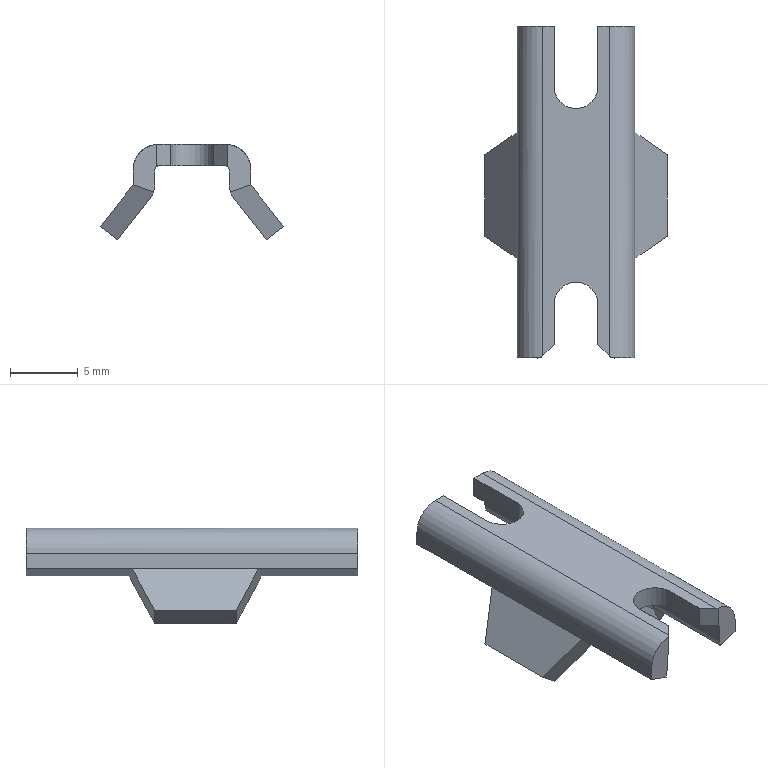Part | STEP file | AC10B-M5_AC3011A Spacer Front Plate(1) | 1 solid | 38 faces | box 13.502 x 24.5 x 7.058 mm | volume 480.167 mm3 | plane 30 | cylinder 8 | commonest cylinder face diameters 3.2 x4 0.6 x2 3.8 x2